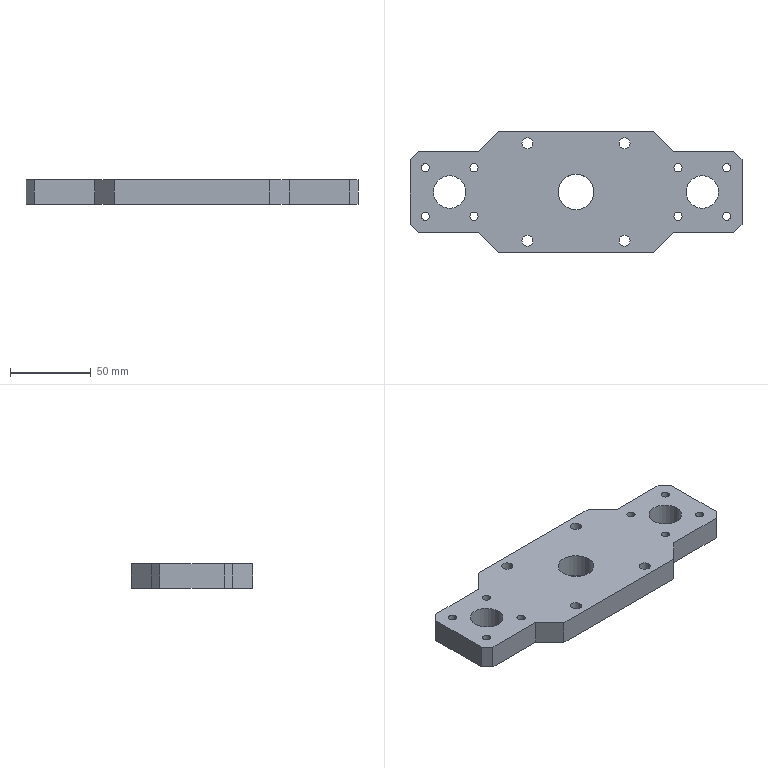Part | STEP file | BU-A01 | 1 solid | 48 faces | box 205 x 75 x 15 mm | volume 173838 mm3 | cylinder 30 | plane 18 | commonest cylinder face diameters 5 x16 6.8 x8 20 x4 22 x2